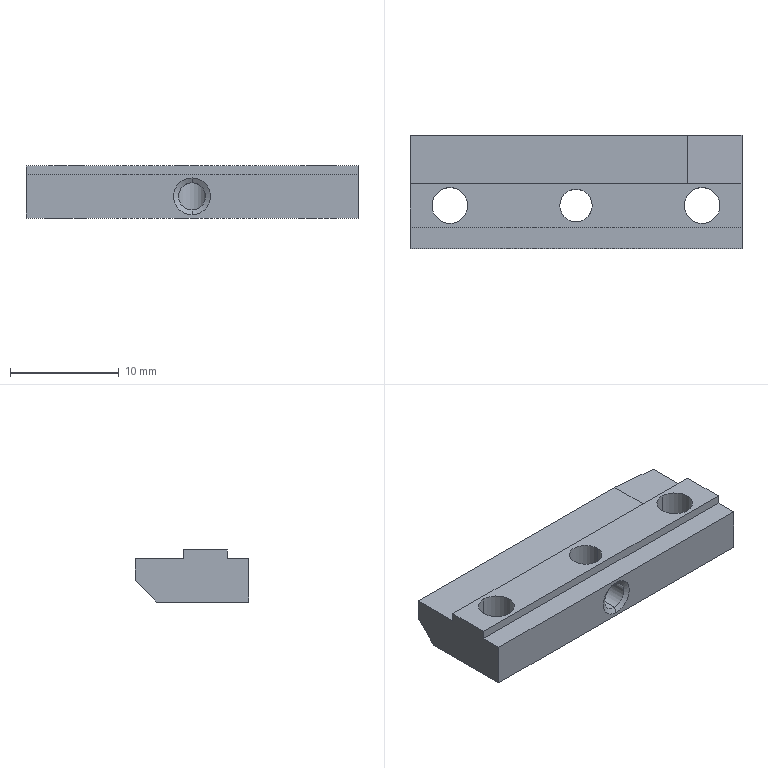Part | NX | 1 solid | 26 faces | box 30.6 x 10.5 x 4.8 mm | volume 1187 mm3 | plane 12 | cylinder 8 | cone 6 | commonest cylinder face diameters 3.3 x4 2.5 x2 3 x2
STEP:
#1=CARTESIAN_POINT('',(-174.8,180.7,-95.7));
#2=VERTEX_POINT('',#1);
#3=CARTESIAN_POINT('',(-174.8,176.706,-95.7));
#4=VERTEX_POINT('',#3);
#5=CARTESIAN_POINT('',(-174.8,178.513,-95.7));
#6=DIRECTION('',(0.,-1.,0.));
#7=VECTOR('',#6,1000.);
#8=LINE('',#5,#7);
#9=EDGE_CURVE('',#2,#4,#8,.T.);
#10=ORIENTED_EDGE('',*,*,#9,.T.);
#11=CARTESIAN_POINT('',(-144.2,176.706,-95.7));
#12=VERTEX_POINT('',#11);
#13=CARTESIAN_POINT('',(-175.,176.706,-95.7));
#14=DIRECTION('',(-1.,0.,0.));
#15=VECTOR('',#14,1000.);
#16=LINE('',#13,#15);
#17=EDGE_CURVE('',#12,#4,#16,.T.);
#18=ORIENTED_EDGE('',*,*,#17,.F.);
#19=CARTESIAN_POINT('',(-144.2,180.7,-95.7));
#20=VERTEX_POINT('',#19);
#21=CARTESIAN_POINT('',(-144.2,178.513,-95.7));
#22=DIRECTION('',(0.,-1.,0.));
#23=VECTOR('',#22,1000.);
#24=LINE('',#21,#23);
#25=EDGE_CURVE('',#20,#12,#24,.T.);
#26=ORIENTED_EDGE('',*,*,#25,.F.);
#27=CARTESIAN_POINT('',(-175.,180.7,-95.7));
#28=DIRECTION('',(1.,0.,0.));
#29=VECTOR('',#28,1000.);
#30=LINE('',#27,#29);
#31=EDGE_CURVE('',#2,#20,#30,.T.);
#32=ORIENTED_EDGE('',*,*,#31,.F.);
#33=EDGE_LOOP('',(#10,#18,#26,#32));
#34=FACE_BOUND('',#33,.T.);
#35=CARTESIAN_POINT('',(-171.125,177.05,-95.7));
#36=VERTEX_POINT('',#35);
#37=CARTESIAN_POINT('',(-171.125,180.35,-95.7));
#38=VERTEX_POINT('',#37);
#39=CARTESIAN_POINT('',(-171.125,178.7,-95.7));
#40=DIRECTION('',(0.,0.,-1.));
#41=DIRECTION('',(0.,1.,0.));
#42=AXIS2_PLACEMENT_3D('',#39,#40,#41);
#43=CIRCLE('',#42,1.65);
#44=EDGE_CURVE('',#36,#38,#43,.T.);
#45=ORIENTED_EDGE('',*,*,#44,.T.);
#46=CARTESIAN_POINT('',(-171.125,178.7,-95.7));
#47=DIRECTION('',(0.,0.,-1.));
#48=DIRECTION('',(0.,1.,0.));
#49=AXIS2_PLACEMENT_3D('',#46,#47,#48);
#50=CIRCLE('',#49,1.65);
#51=EDGE_CURVE('',#38,#36,#50,.T.);
#52=ORIENTED_EDGE('',*,*,#51,.T.);
#53=EDGE_LOOP('',(#45,#52));
#54=FACE_BOUND('',#53,.T.);
#55=CARTESIAN_POINT('',(-158.,178.7,-95.7));
#56=VERTEX_POINT('',#55);
#57=CARTESIAN_POINT('',(-161.,178.7,-95.7));
#58=VERTEX_POINT('',#57);
#59=CARTESIAN_POINT('',(-159.5,178.7,-95.7));
#60=DIRECTION('',(0.,0.,-1.));
#61=DIRECTION('',(-1.,0.,0.));
#62=AXIS2_PLACEMENT_3D('',#59,#60,#61);
#63=CIRCLE('',#62,1.5);
#64=EDGE_CURVE('',#56,#58,#63,.T.);
#65=ORIENTED_EDGE('',*,*,#64,.T.);
#66=CARTESIAN_POINT('',(-159.5,178.7,-95.7));
#67=DIRECTION('',(0.,0.,-1.));
#68=DIRECTION('',(-1.,0.,0.));
#69=AXIS2_PLACEMENT_3D('',#66,#67,#68);
#70=CIRCLE('',#69,1.5);
#71=EDGE_CURVE('',#58,#56,#70,.T.);
#72=ORIENTED_EDGE('',*,*,#71,.T.);
#73=EDGE_LOOP('',(#65,#72));
#74=FACE_BOUND('',#73,.T.);
#75=CARTESIAN_POINT('',(-147.875,177.05,-95.7));
#76=VERTEX_POINT('',#75);
#77=CARTESIAN_POINT('',(-147.875,180.35,-95.7));
#78=VERTEX_POINT('',#77);
#79=CARTESIAN_POINT('',(-147.875,178.7,-95.7));
#80=DIRECTION('',(0.,0.,-1.));
#81=DIRECTION('',(0.,1.,0.));
#82=AXIS2_PLACEMENT_3D('',#79,#80,#81);
#83=CIRCLE('',#82,1.65);
#84=EDGE_CURVE('',#76,#78,#83,.T.);
#85=ORIENTED_EDGE('',*,*,#84,.T.);
#86=CARTESIAN_POINT('',(-147.875,178.7,-95.7));
#87=DIRECTION('',(0.,0.,-1.));
#88=DIRECTION('',(0.,1.,0.));
#89=AXIS2_PLACEMENT_3D('',#86,#87,#88);
#90=CIRCLE('',#89,1.65);
#91=EDGE_CURVE('',#78,#76,#90,.T.);
#92=ORIENTED_EDGE('',*,*,#91,.T.);
#93=EDGE_LOOP('',(#85,#92));
#94=FACE_BOUND('',#93,.T.);
#95=CARTESIAN_POINT('',(-175.,176.707,-95.7));
#96=DIRECTION('',(0.,0.,1.));
#97=DIRECTION('',(1.,0.,0.));
#98=AXIS2_PLACEMENT_3D('',#95,#96,#97);
#99=PLANE('',#98);
#100=ADVANCED_FACE('',(#34,#54,#74,#94),#99,.T.);
#101=CARTESIAN_POINT('',(-174.8,176.7,-96.5));
#102=VERTEX_POINT('',#101);
#103=CARTESIAN_POINT('',(-174.8,176.744,-90.15));
#104=DIRECTION('',(0.,-0.007004,-1.));
#105=VECTOR('',#104,1000.);
#106=LINE('',#103,#105);
#107=EDGE_CURVE('',#4,#102,#106,.T.);
#108=ORIENTED_EDGE('',*,*,#107,.T.);
#109=CARTESIAN_POINT('',(-144.2,176.7,-96.5));
#110=VERTEX_POINT('',#109);
#111=CARTESIAN_POINT('',(-175.,176.7,-96.5));
#112=DIRECTION('',(1.,0.,0.));
#113=VECTOR('',#112,1000.);
#114=LINE('',#111,#113);
#115=EDGE_CURVE('',#102,#110,#114,.T.);
#116=ORIENTED_EDGE('',*,*,#115,.T.);
#117=CARTESIAN_POINT('',(-144.2,176.744,-90.15));
#118=DIRECTION('',(0.,-0.007004,-1.));
#119=VECTOR('',#118,1000.);
#120=LINE('',#117,#119);
#121=EDGE_CURVE('',#12,#110,#120,.T.);
#122=ORIENTED_EDGE('',*,*,#121,.F.);
#123=ORIENTED_EDGE('',*,*,#17,.T.);
#124=EDGE_LOOP('',(#108,#116,#122,#123));
#125=FACE_BOUND('',#124,.T.);
#126=CARTESIAN_POINT('',(-175.,176.7,-96.5));
#127=DIRECTION('',(0.,-1.,0.007004));
#128=DIRECTION('',(-1.,0.,0.));
#129=AXIS2_PLACEMENT_3D('',#126,#127,#128);
#130=PLANE('',#129);
#131=ADVANCED_FACE('',(#125),#130,.T.);
#132=CARTESIAN_POINT('',(-174.8,174.7,-96.5));
#133=VERTEX_POINT('',#132);
#134=CARTESIAN_POINT('',(-174.8,178.513,-96.5));
#135=DIRECTION('',(0.,-1.,0.));
#136=VECTOR('',#135,1000.);
#137=LINE('',#134,#136);
#138=EDGE_CURVE('',#102,#133,#137,.T.);
#139=ORIENTED_EDGE('',*,*,#138,.T.);
#140=CARTESIAN_POINT('',(-144.2,174.7,-96.5));
#141=VERTEX_POINT('',#140);
#142=CARTESIAN_POINT('',(-175.,174.7,-96.5));
#143=DIRECTION('',(1.,0.,0.));
#144=VECTOR('',#143,1000.);
#145=LINE('',#142,#144);
#146=EDGE_CURVE('',#133,#141,#145,.T.);
#147=ORIENTED_EDGE('',*,*,#146,.T.);
#148=CARTESIAN_POINT('',(-144.2,178.513,-96.5));
#149=DIRECTION('',(0.,-1.,0.));
#150=VECTOR('',#149,1000.);
#151=LINE('',#148,#150);
#152=EDGE_CURVE('',#110,#141,#151,.T.);
#153=ORIENTED_EDGE('',*,*,#152,.F.);
#154=ORIENTED_EDGE('',*,*,#115,.F.);
#155=EDGE_LOOP('',(#139,#147,#153,#154));
#156=FACE_BOUND('',#155,.T.);
#157=CARTESIAN_POINT('',(-175.,174.7,-96.5));
#158=DIRECTION('',(0.,0.,1.));
#159=DIRECTION('',(1.,0.,0.));
#160=AXIS2_PLACEMENT_3D('',#157,#158,#159);
#161=PLANE('',#160);
#162=ADVANCED_FACE('',(#156),#161,.T.);
#163=CARTESIAN_POINT('',(-174.8,174.7,-100.5));
#164=VERTEX_POINT('',#163);
#165=CARTESIAN_POINT('',(-174.8,174.7,-90.15));
#166=DIRECTION('',(0.,0.,-1.));
#167=VECTOR('',#166,1000.);
#168=LINE('',#165,#167);
#169=EDGE_CURVE('',#133,#164,#168,.T.);
#170=ORIENTED_EDGE('',*,*,#169,.T.);
#171=CARTESIAN_POINT('',(-144.2,174.7,-100.5));
#172=VERTEX_POINT('',#171);
#173=CARTESIAN_POINT('',(-175.,174.7,-100.5));
#174=DIRECTION('',(1.,0.,0.));
#175=VECTOR('',#174,1000.);
#176=LINE('',#173,#175);
#177=EDGE_CURVE('',#164,#172,#176,.T.);
#178=ORIENTED_EDGE('',*,*,#177,.T.);
#179=CARTESIAN_POINT('',(-144.2,174.7,-90.15));
#180=DIRECTION('',(0.,0.,-1.));
#181=VECTOR('',#180,1000.);
#182=LINE('',#179,#181);
#183=EDGE_CURVE('',#141,#172,#182,.T.);
#184=ORIENTED_EDGE('',*,*,#183,.F.);
#185=ORIENTED_EDGE('',*,*,#146,.F.);
#186=EDGE_LOOP('',(#170,#178,#184,#185));
#187=FACE_BOUND('',#186,.T.);
#188=CARTESIAN_POINT('',(-159.5,174.7,-96.8));
#189=VERTEX_POINT('',#188);
#190=CARTESIAN_POINT('',(-159.5,174.7,-100.2));
#191=VERTEX_POINT('',#190);
#192=CARTESIAN_POINT('',(-159.5,174.7,-98.5));
#193=DIRECTION('',(0.,-1.,0.));
#194=DIRECTION('',(0.,0.,-1.));
#195=AXIS2_PLACEMENT_3D('',#192,#193,#194);
#196=CIRCLE('',#195,1.7);
#197=EDGE_CURVE('',#189,#191,#196,.T.);
#198=ORIENTED_EDGE('',*,*,#197,.F.);
#199=CARTESIAN_POINT('',(-159.5,174.7,-98.5));
#200=DIRECTION('',(0.,-1.,0.));
#201=DIRECTION('',(0.,0.,-1.));
#202=AXIS2_PLACEMENT_3D('',#199,#200,#201);
#203=CIRCLE('',#202,1.7);
#204=EDGE_CURVE('',#191,#189,#203,.T.);
#205=ORIENTED_EDGE('',*,*,#204,.F.);
#206=EDGE_LOOP('',(#198,#205));
#207=FACE_BOUND('',#206,.T.);
#208=CARTESIAN_POINT('',(-175.,174.7,-100.5));
#209=DIRECTION('',(0.,-1.,0.));
#210=DIRECTION('',(-1.,0.,0.));
#211=AXIS2_PLACEMENT_3D('',#208,#209,#210);
#212=PLANE('',#211);
#213=ADVANCED_FACE('',(#187,#207),#212,.T.);
#214=CARTESIAN_POINT('',(-174.8,183.2,-100.5));
#215=VERTEX_POINT('',#214);
#216=CARTESIAN_POINT('',(-144.2,183.2,-100.5));
#217=VERTEX_POINT('',#216);
#218=CARTESIAN_POINT('',(-175.,183.2,-100.5));
#219=DIRECTION('',(1.,0.,0.));
#220=VECTOR('',#219,1000.);
#221=LINE('',#218,#220);
#222=EDGE_CURVE('',#215,#217,#221,.T.);
#223=ORIENTED_EDGE('',*,*,#222,.T.);
#224=CARTESIAN_POINT('',(-144.2,178.513,-100.5));
#225=DIRECTION('',(0.,1.,0.));
#226=VECTOR('',#225,1000.);
#227=LINE('',#224,#226);
#228=EDGE_CURVE('',#172,#217,#227,.T.);
#229=ORIENTED_EDGE('',*,*,#228,.F.);
#230=ORIENTED_EDGE('',*,*,#177,.F.);
#231=CARTESIAN_POINT('',(-174.8,178.513,-100.5));
#232=DIRECTION('',(0.,1.,0.));
#233=VECTOR('',#232,1000.);
#234=LINE('',#231,#233);
#235=EDGE_CURVE('',#164,#215,#234,.T.);
#236=ORIENTED_EDGE('',*,*,#235,.T.);
#237=EDGE_LOOP('',(#223,#229,#230,#236));
#238=FACE_BOUND('',#237,.T.);
#239=CARTESIAN_POINT('',(-147.875,176.85,-100.5));
#240=VERTEX_POINT('',#239);
#241=CARTESIAN_POINT('',(-147.875,180.55,-100.5));
#242=VERTEX_POINT('',#241);
#243=CARTESIAN_POINT('',(-147.875,178.7,-100.5));
#244=DIRECTION('',(0.,0.,-1.));
#245=DIRECTION('',(0.,1.,0.));
#246=AXIS2_PLACEMENT_3D('',#243,#244,#245);
#247=CIRCLE('',#246,1.85);
#248=EDGE_CURVE('',#240,#242,#247,.T.);
#249=ORIENTED_EDGE('',*,*,#248,.F.);
#250=CARTESIAN_POINT('',(-147.875,178.7,-100.5));
#251=DIRECTION('',(0.,0.,-1.));
#252=DIRECTION('',(0.,1.,0.));
#253=AXIS2_PLACEMENT_3D('',#250,#251,#252);
#254=CIRCLE('',#253,1.85);
#255=EDGE_CURVE('',#242,#240,#254,.T.);
#256=ORIENTED_EDGE('',*,*,#255,.F.);
#257=EDGE_LOOP('',(#249,#256));
#258=FACE_BOUND('',#257,.T.);
#259=CARTESIAN_POINT('',(-158.,178.7,-100.5));
#260=VERTEX_POINT('',#259);
#261=CARTESIAN_POINT('',(-161.,178.7,-100.5));
#262=VERTEX_POINT('',#261);
#263=CARTESIAN_POINT('',(-159.5,178.7,-100.5));
#264=DIRECTION('',(0.,0.,-1.));
#265=DIRECTION('',(-1.,0.,0.));
#266=AXIS2_PLACEMENT_3D('',#263,#264,#265);
#267=CIRCLE('',#266,1.5);
#268=EDGE_CURVE('',#260,#262,#267,.T.);
#269=ORIENTED_EDGE('',*,*,#268,.F.);
#270=CARTESIAN_POINT('',(-159.5,178.7,-100.5));
#271=DIRECTION('',(0.,0.,-1.));
#272=DIRECTION('',(-1.,0.,0.));
#273=AXIS2_PLACEMENT_3D('',#270,#271,#272);
#274=CIRCLE('',#273,1.5);
#275=EDGE_CURVE('',#262,#260,#274,.T.);
#276=ORIENTED_EDGE('',*,*,#275,.F.);
#277=EDGE_LOOP('',(#269,#276));
#278=FACE_BOUND('',#277,.T.);
#279=CARTESIAN_POINT('',(-171.125,176.85,-100.5));
#280=VERTEX_POINT('',#279);
#281=CARTESIAN_POINT('',(-171.125,180.55,-100.5));
#282=VERTEX_POINT('',#281);
#283=CARTESIAN_POINT('',(-171.125,178.7,-100.5));
#284=DIRECTION('',(0.,0.,-1.));
#285=DIRECTION('',(0.,1.,0.));
#286=AXIS2_PLACEMENT_3D('',#283,#284,#285);
#287=CIRCLE('',#286,1.85);
#288=EDGE_CURVE('',#280,#282,#287,.T.);
#289=ORIENTED_EDGE('',*,*,#288,.F.);
#290=CARTESIAN_POINT('',(-171.125,178.7,-100.5));
#291=DIRECTION('',(0.,0.,-1.));
#292=DIRECTION('',(0.,1.,0.));
#293=AXIS2_PLACEMENT_3D('',#290,#291,#292);
#294=CIRCLE('',#293,1.85);
#295=EDGE_CURVE('',#282,#280,#294,.T.);
#296=ORIENTED_EDGE('',*,*,#295,.F.);
#297=EDGE_LOOP('',(#289,#296));
#298=FACE_BOUND('',#297,.T.);
#299=CARTESIAN_POINT('',(-175.,182.7,-100.5));
#300=DIRECTION('',(0.,0.,-1.));
#301=DIRECTION('',(-1.,0.,0.));
#302=AXIS2_PLACEMENT_3D('',#299,#300,#301);
#303=PLANE('',#302);
#304=ADVANCED_FACE('',(#238,#258,#278,#298),#303,.T.);
#305=CARTESIAN_POINT('',(-174.8,185.2,-98.5));
#306=VERTEX_POINT('',#305);
#307=CARTESIAN_POINT('',(-174.8,185.2,-96.5));
#308=VERTEX_POINT('',#307);
#309=CARTESIAN_POINT('',(-174.8,185.2,-90.15));
#310=DIRECTION('',(0.,0.,1.));
#311=VECTOR('',#310,1000.);
#312=LINE('',#309,#311);
#313=EDGE_CURVE('',#306,#308,#312,.T.);
#314=ORIENTED_EDGE('',*,*,#313,.T.);
#315=CARTESIAN_POINT('',(-149.2,185.2,-96.5));
#316=VERTEX_POINT('',#315);
#317=CARTESIAN_POINT('',(-175.,185.2,-96.5));
#318=DIRECTION('',(-1.,0.,0.));
#319=VECTOR('',#318,1000.);
#320=LINE('',#317,#319);
#321=EDGE_CURVE('',#316,#308,#320,.T.);
#322=ORIENTED_EDGE('',*,*,#321,.F.);
#323=CARTESIAN_POINT('',(-144.2,185.2,-96.937));
#324=VERTEX_POINT('',#323);
#325=CARTESIAN_POINT('',(-175.,185.2,-94.243));
#326=DIRECTION('',(-0.9962,0.,0.08716));
#327=VECTOR('',#326,1000.);
#328=LINE('',#325,#327);
#329=EDGE_CURVE('',#324,#316,#328,.T.);
#330=ORIENTED_EDGE('',*,*,#329,.F.);
#331=CARTESIAN_POINT('',(-144.2,185.2,-98.5));
#332=VERTEX_POINT('',#331);
#333=CARTESIAN_POINT('',(-144.2,185.2,-90.15));
#334=DIRECTION('',(0.,0.,1.));
#335=VECTOR('',#334,1000.);
#336=LINE('',#333,#335);
#337=EDGE_CURVE('',#332,#324,#336,.T.);
#338=ORIENTED_EDGE('',*,*,#337,.F.);
#339=CARTESIAN_POINT('',(-175.,185.2,-98.5));
#340=DIRECTION('',(1.,0.,0.));
#341=VECTOR('',#340,1000.);
#342=LINE('',#339,#341);
#343=EDGE_CURVE('',#306,#332,#342,.T.);
#344=ORIENTED_EDGE('',*,*,#343,.F.);
#345=EDGE_LOOP('',(#314,#322,#330,#338,#344));
#346=FACE_BOUND('',#345,.T.);
#347=CARTESIAN_POINT('',(-175.,185.2,-96.5));
#348=DIRECTION('',(0.,1.,0.));
#349=DIRECTION('',(1.,0.,0.));
#350=AXIS2_PLACEMENT_3D('',#347,#348,#349);
#351=PLANE('',#350);
#352=ADVANCED_FACE('',(#346),#351,.T.);
#353=CARTESIAN_POINT('',(-174.8,180.7,-96.5));
#354=VERTEX_POINT('',#353);
#355=CARTESIAN_POINT('',(-174.8,178.513,-96.5));
#356=DIRECTION('',(0.,-1.,0.));
#357=VECTOR('',#356,1000.);
#358=LINE('',#355,#357);
#359=EDGE_CURVE('',#308,#354,#358,.T.);
#360=ORIENTED_EDGE('',*,*,#359,.T.);
#361=CARTESIAN_POINT('',(-149.2,180.7,-96.5));
#362=VERTEX_POINT('',#361);
#363=CARTESIAN_POINT('',(-175.,180.7,-96.5));
#364=DIRECTION('',(1.,0.,0.));
#365=VECTOR('',#364,1000.);
#366=LINE('',#363,#365);
#367=EDGE_CURVE('',#354,#362,#366,.T.);
#368=ORIENTED_EDGE('',*,*,#367,.T.);
#369=CARTESIAN_POINT('',(-149.2,182.95,-96.5));
#370=DIRECTION('',(0.,-1.,0.));
#371=VECTOR('',#370,1000.);
#372=LINE('',#369,#371);
#373=EDGE_CURVE('',#316,#362,#372,.T.);
#374=ORIENTED_EDGE('',*,*,#373,.F.);
#375=ORIENTED_EDGE('',*,*,#321,.T.);
#376=EDGE_LOOP('',(#360,#368,#374,#375));
#377=FACE_BOUND('',#376,.T.);
#378=CARTESIAN_POINT('',(-175.,180.7,-96.5));
#379=DIRECTION('',(0.,0.,1.));
#380=DIRECTION('',(1.,0.,0.));
#381=AXIS2_PLACEMENT_3D('',#378,#379,#380);
#382=PLANE('',#381);
#383=ADVANCED_FACE('',(#377),#382,.T.);
#384=CARTESIAN_POINT('',(-174.8,180.7,-90.15));
#385=DIRECTION('',(0.,0.,1.));
#386=VECTOR('',#385,1000.);
#387=LINE('',#384,#386);
#388=EDGE_CURVE('',#354,#2,#387,.T.);
#389=ORIENTED_EDGE('',*,*,#388,.T.);
#390=ORIENTED_EDGE('',*,*,#31,.T.);
#391=CARTESIAN_POINT('',(-144.2,180.7,-96.937));
#392=VERTEX_POINT('',#391);
#393=CARTESIAN_POINT('',(-144.2,180.7,-90.15));
#394=DIRECTION('',(0.,0.,1.));
#395=VECTOR('',#394,1000.);
#396=LINE('',#393,#395);
#397=EDGE_CURVE('',#392,#20,#396,.T.);
#398=ORIENTED_EDGE('',*,*,#397,.F.);
#399=CARTESIAN_POINT('',(-175.,180.7,-94.243));
#400=DIRECTION('',(-0.9962,0.,0.08716));
#401=VECTOR('',#400,1000.);
#402=LINE('',#399,#401);
#403=EDGE_CURVE('',#392,#362,#402,.T.);
#404=ORIENTED_EDGE('',*,*,#403,.T.);
#405=ORIENTED_EDGE('',*,*,#367,.F.);
#406=EDGE_LOOP('',(#389,#390,#398,#404,#405));
#407=FACE_BOUND('',#406,.T.);
#408=CARTESIAN_POINT('',(-175.,180.7,-95.5));
#409=DIRECTION('',(0.,1.,0.));
#410=DIRECTION('',(1.,0.,0.));
#411=AXIS2_PLACEMENT_3D('',#408,#409,#410);
#412=PLANE('',#411);
#413=ADVANCED_FACE('',(#407),#412,.T.);
#414=CARTESIAN_POINT('',(-171.125,177.05,-100.3));
#415=VERTEX_POINT('',#414);
#416=CARTESIAN_POINT('',(-171.125,180.35,-100.3));
#417=VERTEX_POINT('',#416);
#418=CARTESIAN_POINT('',(-171.125,178.7,-100.3));
#419=DIRECTION('',(0.,0.,-1.));
#420=DIRECTION('',(0.,1.,0.));
#421=AXIS2_PLACEMENT_3D('',#418,#419,#420);
#422=CIRCLE('',#421,1.65);
#423=EDGE_CURVE('',#415,#417,#422,.T.);
#424=ORIENTED_EDGE('',*,*,#423,.T.);
#425=CARTESIAN_POINT('',(-171.125,180.35,-100.5));
#426=DIRECTION('',(0.,0.,-1.));
#427=VECTOR('',#426,1000.);
#428=LINE('',#425,#427);
#429=EDGE_CURVE('',#417,#38,#428,.F.);
#430=ORIENTED_EDGE('',*,*,#429,.T.);
#431=ORIENTED_EDGE('',*,*,#44,.F.);
#432=CARTESIAN_POINT('',(-171.125,177.05,-100.5));
#433=DIRECTION('',(0.,0.,-1.));
#434=VECTOR('',#433,1000.);
#435=LINE('',#432,#434);
#436=EDGE_CURVE('',#415,#36,#435,.F.);
#437=ORIENTED_EDGE('',*,*,#436,.F.);
#438=EDGE_LOOP('',(#424,#430,#431,#437));
#439=FACE_BOUND('',#438,.T.);
#440=CARTESIAN_POINT('',(-171.125,178.7,-100.5));
#441=DIRECTION('',(0.,0.,-1.));
#442=DIRECTION('',(0.,1.,0.));
#443=AXIS2_PLACEMENT_3D('',#440,#441,#442);
#444=CYLINDRICAL_SURFACE('',#443,1.65);
#445=ADVANCED_FACE('',(#439),#444,.F.);
#446=ORIENTED_EDGE('',*,*,#423,.F.);
#447=CARTESIAN_POINT('',(-171.125,177.05,-100.3));
#448=DIRECTION('',(0.,-0.7071,-0.7071));
#449=VECTOR('',#448,1000.);
#450=LINE('',#447,#449);
#451=EDGE_CURVE('',#280,#415,#450,.F.);
#452=ORIENTED_EDGE('',*,*,#451,.F.);
#453=ORIENTED_EDGE('',*,*,#288,.T.);
#454=CARTESIAN_POINT('',(-171.125,180.35,-100.3));
#455=DIRECTION('',(0.,0.7071,-0.7071));
#456=VECTOR('',#455,1000.);
#457=LINE('',#454,#456);
#458=EDGE_CURVE('',#282,#417,#457,.F.);
#459=ORIENTED_EDGE('',*,*,#458,.T.);
#460=EDGE_LOOP('',(#446,#452,#453,#459));
#461=FACE_BOUND('',#460,.T.);
#462=CARTESIAN_POINT('',(-171.125,178.7,-100.3));
#463=DIRECTION('',(0.,0.,-1.));
#464=DIRECTION('',(0.,1.,0.));
#465=AXIS2_PLACEMENT_3D('',#462,#463,#464);
#466=CONICAL_SURFACE('',#465,1.65,0.7854);
#467=ADVANCED_FACE('',(#461),#466,.F.);
#468=CARTESIAN_POINT('',(-147.875,177.05,-100.3));
#469=VERTEX_POINT('',#468);
#470=CARTESIAN_POINT('',(-147.875,180.35,-100.3));
#471=VERTEX_POINT('',#470);
#472=CARTESIAN_POINT('',(-147.875,178.7,-100.3));
#473=DIRECTION('',(0.,0.,-1.));
#474=DIRECTION('',(0.,1.,0.));
#475=AXIS2_PLACEMENT_3D('',#472,#473,#474);
#476=CIRCLE('',#475,1.65);
#477=EDGE_CURVE('',#469,#471,#476,.T.);
#478=ORIENTED_EDGE('',*,*,#477,.T.);
#479=CARTESIAN_POINT('',(-147.875,180.35,-100.5));
#480=DIRECTION('',(0.,0.,-1.));
#481=VECTOR('',#480,1000.);
#482=LINE('',#479,#481);
#483=EDGE_CURVE('',#471,#78,#482,.F.);
#484=ORIENTED_EDGE('',*,*,#483,.T.);
#485=ORIENTED_EDGE('',*,*,#84,.F.);
#486=CARTESIAN_POINT('',(-147.875,177.05,-100.5));
#487=DIRECTION('',(0.,0.,-1.));
#488=VECTOR('',#487,1000.);
#489=LINE('',#486,#488);
#490=EDGE_CURVE('',#469,#76,#489,.F.);
#491=ORIENTED_EDGE('',*,*,#490,.F.);
#492=EDGE_LOOP('',(#478,#484,#485,#491));
#493=FACE_BOUND('',#492,.T.);
#494=CARTESIAN_POINT('',(-147.875,178.7,-100.5));
#495=DIRECTION('',(0.,0.,-1.));
#496=DIRECTION('',(0.,1.,0.));
#497=AXIS2_PLACEMENT_3D('',#494,#495,#496);
#498=CYLINDRICAL_SURFACE('',#497,1.65);
#499=ADVANCED_FACE('',(#493),#498,.F.);
#500=ORIENTED_EDGE('',*,*,#477,.F.);
#501=CARTESIAN_POINT('',(-147.875,177.05,-100.3));
#502=DIRECTION('',(0.,-0.7071,-0.7071));
#503=VECTOR('',#502,1000.);
#504=LINE('',#501,#503);
#505=EDGE_CURVE('',#240,#469,#504,.F.);
#506=ORIENTED_EDGE('',*,*,#505,.F.);
#507=ORIENTED_EDGE('',*,*,#248,.T.);
#508=CARTESIAN_POINT('',(-147.875,180.35,-100.3));
#509=DIRECTION('',(0.,0.7071,-0.7071));
#510=VECTOR('',#509,1000.);
#511=LINE('',#508,#510);
#512=EDGE_CURVE('',#242,#471,#511,.F.);
#513=ORIENTED_EDGE('',*,*,#512,.T.);
#514=EDGE_LOOP('',(#500,#506,#507,#513));
#515=FACE_BOUND('',#514,.T.);
#516=CARTESIAN_POINT('',(-147.875,178.7,-100.3));
#517=DIRECTION('',(0.,0.,-1.));
#518=DIRECTION('',(0.,1.,0.));
#519=AXIS2_PLACEMENT_3D('',#516,#517,#518);
#520=CONICAL_SURFACE('',#519,1.65,0.7854);
#521=ADVANCED_FACE('',(#515),#520,.F.);
#522=ORIENTED_EDGE('',*,*,#64,.F.);
#523=CARTESIAN_POINT('',(-158.,178.7,-95.22));
#524=DIRECTION('',(0.,0.,-1.));
#525=VECTOR('',#524,1000.);
#526=LINE('',#523,#525);
#527=EDGE_CURVE('',#260,#56,#526,.F.);
#528=ORIENTED_EDGE('',*,*,#527,.F.);
#529=ORIENTED_EDGE('',*,*,#268,.T.);
#530=CARTESIAN_POINT('',(-161.,178.7,-95.22));
#531=DIRECTION('',(0.,0.,-1.));
#532=VECTOR('',#531,1000.);
#533=LINE('',#530,#532);
#534=EDGE_CURVE('',#262,#58,#533,.F.);
#535=ORIENTED_EDGE('',*,*,#534,.T.);
#536=EDGE_LOOP('',(#522,#528,#529,#535));
#537=FACE_BOUND('',#536,.T.);
#538=CARTESIAN_POINT('',(-159.5,177.2,-97.25));
#539=VERTEX_POINT('',#538);
#540=CARTESIAN_POINT('',(-160.75,177.871,-98.5));
#541=VERTEX_POINT('',#540);
#542=CARTESIAN_POINT('',(-159.5,177.2,-97.25));
#543=CARTESIAN_POINT('',(-159.522,177.2,-97.25));
#544=CARTESIAN_POINT('',(-159.544,177.2,-97.251));
#545=CARTESIAN_POINT('',(-159.566,177.201,-97.252));
#546=CARTESIAN_POINT('',(-159.587,177.202,-97.253));
#547=CARTESIAN_POINT('',(-159.609,177.204,-97.255));
#548=CARTESIAN_POINT('',(-159.631,177.206,-97.257));
#549=CARTESIAN_POINT('',(-159.653,177.208,-97.259));
#550=CARTESIAN_POINT('',(-159.674,177.21,-97.262));
#551=CARTESIAN_POINT('',(-159.696,177.213,-97.265));
#552=CARTESIAN_POINT('',(-159.717,177.216,-97.269));
#553=CARTESIAN_POINT('',(-159.738,177.219,-97.273));
#554=CARTESIAN_POINT('',(-159.759,177.223,-97.277));
#555=CARTESIAN_POINT('',(-159.78,177.226,-97.282));
#556=CARTESIAN_POINT('',(-159.801,177.23,-97.287));
#557=CARTESIAN_POINT('',(-159.822,177.235,-97.292));
#558=CARTESIAN_POINT('',(-159.842,177.239,-97.298));
#559=CARTESIAN_POINT('',(-159.863,177.244,-97.304));
#560=CARTESIAN_POINT('',(-159.883,177.25,-97.31));
#561=CARTESIAN_POINT('',(-159.903,177.255,-97.317));
#562=CARTESIAN_POINT('',(-159.923,177.261,-97.324));
#563=CARTESIAN_POINT('',(-159.943,177.267,-97.331));
#564=CARTESIAN_POINT('',(-159.962,177.273,-97.338));
#565=CARTESIAN_POINT('',(-159.982,177.279,-97.346));
#566=CARTESIAN_POINT('',(-160.001,177.286,-97.355));
#567=CARTESIAN_POINT('',(-160.02,177.293,-97.363));
#568=CARTESIAN_POINT('',(-160.039,177.3,-97.372));
#569=CARTESIAN_POINT('',(-160.057,177.307,-97.381));
#570=CARTESIAN_POINT('',(-160.076,177.315,-97.39));
#571=CARTESIAN_POINT('',(-160.094,177.322,-97.4));
#572=CARTESIAN_POINT('',(-160.111,177.33,-97.41));
#573=CARTESIAN_POINT('',(-160.147,177.346,-97.429));
#574=CARTESIAN_POINT('',(-160.181,177.363,-97.451));
#575=CARTESIAN_POINT('',(-160.214,177.381,-97.474));
#576=CARTESIAN_POINT('',(-160.246,177.398,-97.496));
#577=CARTESIAN_POINT('',(-160.278,177.417,-97.521));
#578=CARTESIAN_POINT('',(-160.308,177.436,-97.546));
#579=CARTESIAN_POINT('',(-160.338,177.455,-97.572));
#580=CARTESIAN_POINT('',(-160.367,177.475,-97.598));
#581=CARTESIAN_POINT('',(-160.394,177.495,-97.626));
#582=CARTESIAN_POINT('',(-160.407,177.505,-97.64));
#583=CARTESIAN_POINT('',(-160.421,177.516,-97.654));
#584=CARTESIAN_POINT('',(-160.433,177.526,-97.669));
#585=CARTESIAN_POINT('',(-160.446,177.536,-97.683));
#586=CARTESIAN_POINT('',(-160.459,177.546,-97.698));
#587=CARTESIAN_POINT('',(-160.471,177.556,-97.712));
#588=CARTESIAN_POINT('',(-160.483,177.567,-97.727));
#589=CARTESIAN_POINT('',(-160.495,177.577,-97.743));
#590=CARTESIAN_POINT('',(-160.506,177.587,-97.758));
#591=CARTESIAN_POINT('',(-160.517,177.598,-97.774));
#592=CARTESIAN_POINT('',(-160.529,177.608,-97.789));
#593=CARTESIAN_POINT('',(-160.539,177.618,-97.805));
#594=CARTESIAN_POINT('',(-160.55,177.629,-97.821));
#595=CARTESIAN_POINT('',(-160.56,177.639,-97.838));
#596=CARTESIAN_POINT('',(-160.57,177.649,-97.854));
#597=CARTESIAN_POINT('',(-160.58,177.659,-97.871));
#598=CARTESIAN_POINT('',(-160.59,177.669,-97.888));
#599=CARTESIAN_POINT('',(-160.599,177.679,-97.905));
#600=CARTESIAN_POINT('',(-160.609,177.689,-97.922));
#601=CARTESIAN_POINT('',(-160.617,177.699,-97.94));
#602=CARTESIAN_POINT('',(-160.626,177.709,-97.957));
#603=CARTESIAN_POINT('',(-160.634,177.719,-97.975));
#604=CARTESIAN_POINT('',(-160.643,177.728,-97.993));
#605=CARTESIAN_POINT('',(-160.65,177.737,-98.011));
#606=CARTESIAN_POINT('',(-160.658,177.747,-98.029));
#607=CARTESIAN_POINT('',(-160.665,177.756,-98.048));
#608=CARTESIAN_POINT('',(-160.672,177.764,-98.066));
#609=CARTESIAN_POINT('',(-160.679,177.773,-98.085));
#610=CARTESIAN_POINT('',(-160.686,177.781,-98.104));
#611=CARTESIAN_POINT('',(-160.692,177.789,-98.123));
#612=CARTESIAN_POINT('',(-160.698,177.797,-98.143));
#613=CARTESIAN_POINT('',(-160.704,177.805,-98.163));
#614=CARTESIAN_POINT('',(-160.709,177.812,-98.183));
#615=CARTESIAN_POINT('',(-160.714,177.819,-98.203));
#616=CARTESIAN_POINT('',(-160.719,177.826,-98.223));
#617=CARTESIAN_POINT('',(-160.723,177.832,-98.243));
#618=CARTESIAN_POINT('',(-160.728,177.838,-98.264));
#619=CARTESIAN_POINT('',(-160.732,177.844,-98.285));
#620=CARTESIAN_POINT('',(-160.735,177.848,-98.306));
#621=CARTESIAN_POINT('',(-160.738,177.853,-98.327));
#622=CARTESIAN_POINT('',(-160.741,177.857,-98.348));
#623=CARTESIAN_POINT('',(-160.743,177.861,-98.37));
#624=CARTESIAN_POINT('',(-160.745,177.864,-98.391));
#625=CARTESIAN_POINT('',(-160.747,177.867,-98.413));
#626=CARTESIAN_POINT('',(-160.748,177.868,-98.434));
#627=CARTESIAN_POINT('',(-160.749,177.869,-98.445));
#628=CARTESIAN_POINT('',(-160.749,177.87,-98.456));
#629=CARTESIAN_POINT('',(-160.75,177.87,-98.467));
#630=CARTESIAN_POINT('',(-160.75,177.871,-98.478));
#631=CARTESIAN_POINT('',(-160.75,177.871,-98.489));
#632=CARTESIAN_POINT('',(-160.75,177.871,-98.5));
#633=B_SPLINE_CURVE_WITH_KNOTS('',3,(#542,#543,#544,#545,#546,#547,#548,#549,#550,#551,#552,#553,#554,#555,#556,#557,#558,#559,#560,#561,#562,#563,#564,#565,#566,#567,#568,#569,#570,#571,#572,#573,#574,#575,#576,#577,#578,#579,#580,#581,#582,#583,#584,#585,#586,#587,#588,#589,#590,#591,#592,#593,#594,#595,#596,#597,#598,#599,#600,#601,#602,#603,#604,#605,#606,#607,#608,#609,#610,#611,#612,#613,#614,#615,#616,#617,#618,#619,#620,#621,#622,#623,#624,#625,#626,#627,#628,#629,#630,#631,#632),.UNSPECIFIED.,.F.,.F.,(4,3,3,3,3,3,3,3,3,3,3,3,3,3,3,3,3,3,3,3,3,3,3,3,3,3,3,3,3,3,4),(0.,0.0656,0.1313,0.197,0.2625,0.3278,0.3933,0.459,0.5247,0.5903,0.6557,0.7865,0.9179,1.049,1.115,1.18,1.246,1.311,1.377,1.443,1.508,1.574,1.639,1.705,1.77,1.836,1.902,1.967,2.032,2.065,2.098),.UNSPECIFIED.);
#634=EDGE_CURVE('',#539,#541,#633,.T.);
#635=ORIENTED_EDGE('',*,*,#634,.T.);
#636=CARTESIAN_POINT('',(-159.5,177.2,-99.75));
#637=VERTEX_POINT('',#636);
#638=CARTESIAN_POINT('',(-160.75,177.871,-98.5));
#639=CARTESIAN_POINT('',(-160.75,177.871,-98.511));
#640=CARTESIAN_POINT('',(-160.75,177.871,-98.522));
#641=CARTESIAN_POINT('',(-160.75,177.87,-98.533));
#642=CARTESIAN_POINT('',(-160.749,177.87,-98.544));
#643=CARTESIAN_POINT('',(-160.749,177.869,-98.555));
#644=CARTESIAN_POINT('',(-160.748,177.868,-98.566));
#645=CARTESIAN_POINT('',(-160.748,177.867,-98.577));
#646=CARTESIAN_POINT('',(-160.747,177.866,-98.588));
#647=CARTESIAN_POINT('',(-160.746,177.865,-98.598));
#648=CARTESIAN_POINT('',(-160.745,177.864,-98.609));
#649=CARTESIAN_POINT('',(-160.744,177.862,-98.62));
#650=CARTESIAN_POINT('',(-160.743,177.861,-98.631));
#651=CARTESIAN_POINT('',(-160.741,177.857,-98.652));
#652=CARTESIAN_POINT('',(-160.738,177.853,-98.673));
#653=CARTESIAN_POINT('',(-160.735,177.848,-98.694));
#654=CARTESIAN_POINT('',(-160.732,177.844,-98.715));
#655=CARTESIAN_POINT('',(-160.728,177.838,-98.736));
#656=CARTESIAN_POINT('',(-160.723,177.832,-98.757));
#657=CARTESIAN_POINT('',(-160.719,177.826,-98.777));
#658=CARTESIAN_POINT('',(-160.714,177.819,-98.797));
#659=CARTESIAN_POINT('',(-160.709,177.812,-98.817));
#660=CARTESIAN_POINT('',(-160.704,177.805,-98.837));
#661=CARTESIAN_POINT('',(-160.698,177.797,-98.857));
#662=CARTESIAN_POINT('',(-160.692,177.789,-98.877));
#663=CARTESIAN_POINT('',(-160.686,177.781,-98.896));
#664=CARTESIAN_POINT('',(-160.679,177.773,-98.915));
#665=CARTESIAN_POINT('',(-160.672,177.764,-98.934));
#666=CARTESIAN_POINT('',(-160.665,177.756,-98.952));
#667=CARTESIAN_POINT('',(-160.658,177.747,-98.971));
#668=CARTESIAN_POINT('',(-160.65,177.737,-98.989));
#669=CARTESIAN_POINT('',(-160.643,177.728,-99.007));
#670=CARTESIAN_POINT('',(-160.635,177.719,-99.025));
#671=CARTESIAN_POINT('',(-160.626,177.709,-99.043));
#672=CARTESIAN_POINT('',(-160.618,177.699,-99.06));
#673=CARTESIAN_POINT('',(-160.609,177.69,-99.078));
#674=CARTESIAN_POINT('',(-160.599,177.68,-99.095));
#675=CARTESIAN_POINT('',(-160.59,177.67,-99.112));
#676=CARTESIAN_POINT('',(-160.581,177.659,-99.129));
#677=CARTESIAN_POINT('',(-160.571,177.649,-99.145));
#678=CARTESIAN_POINT('',(-160.561,177.639,-99.162));
#679=CARTESIAN_POINT('',(-160.55,177.629,-99.178));
#680=CARTESIAN_POINT('',(-160.539,177.619,-99.194));
#681=CARTESIAN_POINT('',(-160.529,177.608,-99.21));
#682=CARTESIAN_POINT('',(-160.518,177.598,-99.226));
#683=CARTESIAN_POINT('',(-160.506,177.588,-99.242));
#684=CARTESIAN_POINT('',(-160.495,177.577,-99.257));
#685=CARTESIAN_POINT('',(-160.483,177.567,-99.272));
#686=CARTESIAN_POINT('',(-160.471,177.557,-99.287));
#687=CARTESIAN_POINT('',(-160.447,177.536,-99.317));
#688=CARTESIAN_POINT('',(-160.421,177.516,-99.346));
#689=CARTESIAN_POINT('',(-160.394,177.496,-99.374));
#690=CARTESIAN_POINT('',(-160.367,177.475,-99.401));
#691=CARTESIAN_POINT('',(-160.338,177.456,-99.428));
#692=CARTESIAN_POINT('',(-160.308,177.436,-99.454));
#693=CARTESIAN_POINT('',(-160.278,177.417,-99.479));
#694=CARTESIAN_POINT('',(-160.247,177.398,-99.503));
#695=CARTESIAN_POINT('',(-160.214,177.381,-99.526));
#696=CARTESIAN_POINT('',(-160.181,177.363,-99.549));
#697=CARTESIAN_POINT('',(-160.147,177.346,-99.57));
#698=CARTESIAN_POINT('',(-160.111,177.33,-99.59));
#699=CARTESIAN_POINT('',(-160.076,177.314,-99.61));
#700=CARTESIAN_POINT('',(-160.039,177.3,-99.628));
#701=CARTESIAN_POINT('',(-160.001,177.286,-99.645));
#702=CARTESIAN_POINT('',(-159.982,177.279,-99.653));
#703=CARTESIAN_POINT('',(-159.963,177.273,-99.661));
#704=CARTESIAN_POINT('',(-159.943,177.267,-99.669));
#705=CARTESIAN_POINT('',(-159.923,177.261,-99.676));
#706=CARTESIAN_POINT('',(-159.903,177.255,-99.683));
#707=CARTESIAN_POINT('',(-159.883,177.25,-99.69));
#708=CARTESIAN_POINT('',(-159.863,177.244,-99.696));
#709=CARTESIAN_POINT('',(-159.842,177.239,-99.702));
#710=CARTESIAN_POINT('',(-159.822,177.235,-99.708));
#711=CARTESIAN_POINT('',(-159.801,177.23,-99.713));
#712=CARTESIAN_POINT('',(-159.78,177.226,-99.718));
#713=CARTESIAN_POINT('',(-159.759,177.223,-99.723));
#714=CARTESIAN_POINT('',(-159.738,177.219,-99.727));
#715=CARTESIAN_POINT('',(-159.717,177.216,-99.731));
#716=CARTESIAN_POINT('',(-159.695,177.213,-99.735));
#717=CARTESIAN_POINT('',(-159.674,177.21,-99.738));
#718=CARTESIAN_POINT('',(-159.653,177.208,-99.741));
#719=CARTESIAN_POINT('',(-159.631,177.206,-99.743));
#720=CARTESIAN_POINT('',(-159.609,177.204,-99.745));
#721=CARTESIAN_POINT('',(-159.587,177.202,-99.747));
#722=CARTESIAN_POINT('',(-159.566,177.201,-99.748));
#723=CARTESIAN_POINT('',(-159.544,177.2,-99.749));
#724=CARTESIAN_POINT('',(-159.522,177.2,-99.75));
#725=CARTESIAN_POINT('',(-159.5,177.2,-99.75));
#726=B_SPLINE_CURVE_WITH_KNOTS('',3,(#638,#639,#640,#641,#642,#643,#644,#645,#646,#647,#648,#649,#650,#651,#652,#653,#654,#655,#656,#657,#658,#659,#660,#661,#662,#663,#664,#665,#666,#667,#668,#669,#670,#671,#672,#673,#674,#675,#676,#677,#678,#679,#680,#681,#682,#683,#684,#685,#686,#687,#688,#689,#690,#691,#692,#693,#694,#695,#696,#697,#698,#699,#700,#701,#702,#703,#704,#705,#706,#707,#708,#709,#710,#711,#712,#713,#714,#715,#716,#717,#718,#719,#720,#721,#722,#723,#724,#725),.UNSPECIFIED.,.F.,.F.,(4,3,3,3,3,3,3,3,3,3,3,3,3,3,3,3,3,3,3,3,3,3,3,3,3,3,3,3,3,4),(0.,0.03292,0.06582,0.09866,0.1314,0.1967,0.2621,0.3278,0.3934,0.4588,0.5241,0.5895,0.6551,0.7207,0.7863,0.8519,0.9173,1.048,1.18,1.311,1.442,1.573,1.639,1.705,1.77,1.836,1.901,1.967,2.032,2.098),.UNSPECIFIED.);
#727=EDGE_CURVE('',#541,#637,#726,.T.);
#728=ORIENTED_EDGE('',*,*,#727,.T.);
#729=CARTESIAN_POINT('',(-159.5,177.2,-99.75));
#730=CARTESIAN_POINT('',(-159.472,177.2,-99.75));
#731=CARTESIAN_POINT('',(-159.445,177.201,-99.749));
#732=CARTESIAN_POINT('',(-159.417,177.202,-99.747));
#733=CARTESIAN_POINT('',(-159.402,177.203,-99.746));
#734=CARTESIAN_POINT('',(-159.387,177.204,-99.745));
#735=CARTESIAN_POINT('',(-159.372,177.205,-99.743));
#736=CARTESIAN_POINT('',(-159.357,177.207,-99.742));
#737=CARTESIAN_POINT('',(-159.342,177.208,-99.74));
#738=CARTESIAN_POINT('',(-159.327,177.21,-99.738));
#739=CARTESIAN_POINT('',(-159.297,177.213,-99.734));
#740=CARTESIAN_POINT('',(-159.268,177.218,-99.729));
#741=CARTESIAN_POINT('',(-159.239,177.223,-99.722));
#742=CARTESIAN_POINT('',(-159.209,177.228,-99.716));
#743=CARTESIAN_POINT('',(-159.18,177.234,-99.709));
#744=CARTESIAN_POINT('',(-159.152,177.241,-99.701));
#745=CARTESIAN_POINT('',(-159.123,177.248,-99.692));
#746=CARTESIAN_POINT('',(-159.096,177.255,-99.683));
#747=CARTESIAN_POINT('',(-159.068,177.263,-99.673));
#748=CARTESIAN_POINT('',(-159.041,177.272,-99.663));
#749=CARTESIAN_POINT('',(-159.014,177.281,-99.652));
#750=CARTESIAN_POINT('',(-158.988,177.29,-99.64));
#751=CARTESIAN_POINT('',(-158.962,177.3,-99.629));
#752=CARTESIAN_POINT('',(-158.936,177.31,-99.616));
#753=CARTESIAN_POINT('',(-158.911,177.32,-99.603));
#754=CARTESIAN_POINT('',(-158.886,177.331,-99.589));
#755=CARTESIAN_POINT('',(-158.862,177.342,-99.575));
#756=CARTESIAN_POINT('',(-158.838,177.354,-99.56));
#757=CARTESIAN_POINT('',(-158.814,177.366,-99.545));
#758=CARTESIAN_POINT('',(-158.791,177.378,-99.53));
#759=CARTESIAN_POINT('',(-158.768,177.391,-99.514));
#760=CARTESIAN_POINT('',(-158.743,177.404,-99.496));
#761=CARTESIAN_POINT('',(-158.719,177.419,-99.477));
#762=CARTESIAN_POINT('',(-158.696,177.434,-99.457));
#763=CARTESIAN_POINT('',(-158.673,177.448,-99.438));
#764=CARTESIAN_POINT('',(-158.651,177.463,-99.418));
#765=CARTESIAN_POINT('',(-158.629,177.479,-99.397));
#766=CARTESIAN_POINT('',(-158.608,177.494,-99.376));
#767=CARTESIAN_POINT('',(-158.587,177.51,-99.354));
#768=CARTESIAN_POINT('',(-158.567,177.526,-99.332));
#769=CARTESIAN_POINT('',(-158.547,177.541,-99.309));
#770=CARTESIAN_POINT('',(-158.528,177.557,-99.286));
#771=CARTESIAN_POINT('',(-158.51,177.573,-99.263));
#772=CARTESIAN_POINT('',(-158.491,177.589,-99.239));
#773=CARTESIAN_POINT('',(-158.474,177.606,-99.215));
#774=CARTESIAN_POINT('',(-158.458,177.621,-99.19));
#775=CARTESIAN_POINT('',(-158.441,177.637,-99.165));
#776=CARTESIAN_POINT('',(-158.425,177.653,-99.139));
#777=CARTESIAN_POINT('',(-158.411,177.669,-99.113));
#778=CARTESIAN_POINT('',(-158.403,177.677,-99.1));
#779=CARTESIAN_POINT('',(-158.396,177.684,-99.087));
#780=CARTESIAN_POINT('',(-158.389,177.692,-99.074));
#781=CARTESIAN_POINT('',(-158.382,177.699,-99.06));
#782=CARTESIAN_POINT('',(-158.376,177.707,-99.047));
#783=CARTESIAN_POINT('',(-158.369,177.714,-99.033));
#784=CARTESIAN_POINT('',(-158.356,177.729,-99.006));
#785=CARTESIAN_POINT('',(-158.344,177.743,-98.978));
#786=CARTESIAN_POINT('',(-158.333,177.757,-98.949));
#787=CARTESIAN_POINT('',(-158.327,177.765,-98.932));
#788=CARTESIAN_POINT('',(-158.321,177.773,-98.915));
#789=CARTESIAN_POINT('',(-158.315,177.781,-98.897));
#790=CARTESIAN_POINT('',(-158.309,177.788,-98.88));
#791=CARTESIAN_POINT('',(-158.303,177.795,-98.862));
#792=CARTESIAN_POINT('',(-158.298,177.802,-98.844));
#793=CARTESIAN_POINT('',(-158.288,177.816,-98.808));
#794=CARTESIAN_POINT('',(-158.279,177.828,-98.772));
#795=CARTESIAN_POINT('',(-158.272,177.838,-98.734));
#796=CARTESIAN_POINT('',(-158.269,177.844,-98.715));
#797=CARTESIAN_POINT('',(-158.265,177.848,-98.696));
#798=CARTESIAN_POINT('',(-158.263,177.852,-98.677));
#799=CARTESIAN_POINT('',(-158.26,177.856,-98.658));
#800=CARTESIAN_POINT('',(-158.258,177.86,-98.638));
#801=CARTESIAN_POINT('',(-158.256,177.862,-98.619));
#802=CARTESIAN_POINT('',(-158.254,177.865,-98.599));
#803=CARTESIAN_POINT('',(-158.252,177.867,-98.579));
#804=CARTESIAN_POINT('',(-158.251,177.869,-98.56));
#805=CARTESIAN_POINT('',(-158.25,177.87,-98.54));
#806=CARTESIAN_POINT('',(-158.25,177.871,-98.52));
#807=CARTESIAN_POINT('',(-158.25,177.871,-98.5));
#808=CARTESIAN_POINT('',(-158.25,177.871,-98.481));
#809=CARTESIAN_POINT('',(-158.25,177.87,-98.461));
#810=CARTESIAN_POINT('',(-158.251,177.869,-98.441));
#811=CARTESIAN_POINT('',(-158.252,177.867,-98.421));
#812=CARTESIAN_POINT('',(-158.254,177.865,-98.402));
#813=CARTESIAN_POINT('',(-158.256,177.862,-98.382));
#814=CARTESIAN_POINT('',(-158.257,177.86,-98.362));
#815=CARTESIAN_POINT('',(-158.26,177.856,-98.343));
#816=CARTESIAN_POINT('',(-158.263,177.852,-98.324));
#817=CARTESIAN_POINT('',(-158.265,177.848,-98.304));
#818=CARTESIAN_POINT('',(-158.268,177.844,-98.285));
#819=CARTESIAN_POINT('',(-158.272,177.839,-98.266));
#820=CARTESIAN_POINT('',(-158.274,177.836,-98.257));
#821=CARTESIAN_POINT('',(-158.276,177.833,-98.248));
#822=CARTESIAN_POINT('',(-158.278,177.831,-98.238));
#823=CARTESIAN_POINT('',(-158.28,177.828,-98.229));
#824=CARTESIAN_POINT('',(-158.282,177.825,-98.22));
#825=CARTESIAN_POINT('',(-158.284,177.822,-98.211));
#826=CARTESIAN_POINT('',(-158.288,177.816,-98.192));
#827=CARTESIAN_POINT('',(-158.293,177.809,-98.174));
#828=CARTESIAN_POINT('',(-158.298,177.802,-98.156));
#829=CARTESIAN_POINT('',(-158.303,177.796,-98.139));
#830=CARTESIAN_POINT('',(-158.309,177.788,-98.121));
#831=CARTESIAN_POINT('',(-158.315,177.781,-98.103));
#832=CARTESIAN_POINT('',(-158.32,177.773,-98.086));
#833=CARTESIAN_POINT('',(-158.327,177.766,-98.069));
#834=CARTESIAN_POINT('',(-158.333,177.757,-98.052));
#835=CARTESIAN_POINT('',(-158.344,177.744,-98.023));
#836=CARTESIAN_POINT('',(-158.356,177.729,-97.995));
#837=CARTESIAN_POINT('',(-158.369,177.715,-97.967));
#838=CARTESIAN_POINT('',(-158.376,177.707,-97.954));
#839=CARTESIAN_POINT('',(-158.382,177.7,-97.94));
#840=CARTESIAN_POINT('',(-158.389,177.692,-97.927));
#841=CARTESIAN_POINT('',(-158.396,177.684,-97.914));
#842=CARTESIAN_POINT('',(-158.403,177.677,-97.9));
#843=CARTESIAN_POINT('',(-158.41,177.669,-97.887));
#844=CARTESIAN_POINT('',(-158.425,177.654,-97.861));
#845=CARTESIAN_POINT('',(-158.441,177.638,-97.836));
#846=CARTESIAN_POINT('',(-158.457,177.622,-97.811));
#847=CARTESIAN_POINT('',(-158.474,177.606,-97.786));
#848=CARTESIAN_POINT('',(-158.491,177.59,-97.762));
#849=CARTESIAN_POINT('',(-158.509,177.574,-97.738));
#850=CARTESIAN_POINT('',(-158.527,177.558,-97.714));
#851=CARTESIAN_POINT('',(-158.547,177.542,-97.691));
#852=CARTESIAN_POINT('',(-158.566,177.526,-97.669));
#853=CARTESIAN_POINT('',(-158.586,177.51,-97.646));
#854=CARTESIAN_POINT('',(-158.607,177.494,-97.625));
#855=CARTESIAN_POINT('',(-158.629,177.479,-97.604));
#856=CARTESIAN_POINT('',(-158.65,177.464,-97.583));
#857=CARTESIAN_POINT('',(-158.673,177.448,-97.562));
#858=CARTESIAN_POINT('',(-158.696,177.434,-97.543));
#859=CARTESIAN_POINT('',(-158.707,177.426,-97.533));
#860=CARTESIAN_POINT('',(-158.719,177.419,-97.524));
#861=CARTESIAN_POINT('',(-158.731,177.412,-97.514));
#862=CARTESIAN_POINT('',(-158.743,177.405,-97.505));
#863=CARTESIAN_POINT('',(-158.756,177.398,-97.496));
#864=CARTESIAN_POINT('',(-158.768,177.391,-97.487));
#865=CARTESIAN_POINT('',(-158.79,177.378,-97.471));
#866=CARTESIAN_POINT('',(-158.814,177.366,-97.455));
#867=CARTESIAN_POINT('',(-158.837,177.354,-97.44));
#868=CARTESIAN_POINT('',(-158.861,177.343,-97.425));
#869=CARTESIAN_POINT('',(-158.886,177.331,-97.411));
#870=CARTESIAN_POINT('',(-158.911,177.321,-97.398));
#871=CARTESIAN_POINT('',(-158.936,177.31,-97.384));
#872=CARTESIAN_POINT('',(-158.962,177.3,-97.372));
#873=CARTESIAN_POINT('',(-158.988,177.29,-97.36));
#874=CARTESIAN_POINT('',(-159.014,177.281,-97.348));
#875=CARTESIAN_POINT('',(-159.041,177.272,-97.337));
#876=CARTESIAN_POINT('',(-159.068,177.264,-97.327));
#877=CARTESIAN_POINT('',(-159.082,177.259,-97.322));
#878=CARTESIAN_POINT('',(-159.095,177.256,-97.317));
#879=CARTESIAN_POINT('',(-159.109,177.252,-97.313));
#880=CARTESIAN_POINT('',(-159.123,177.248,-97.308));
#881=CARTESIAN_POINT('',(-159.137,177.244,-97.304));
#882=CARTESIAN_POINT('',(-159.151,177.241,-97.3));
#883=CARTESIAN_POINT('',(-159.18,177.234,-97.291));
#884=CARTESIAN_POINT('',(-159.209,177.228,-97.284));
#885=CARTESIAN_POINT('',(-159.238,177.223,-97.278));
#886=CARTESIAN_POINT('',(-159.253,177.22,-97.275));
#887=CARTESIAN_POINT('',(-159.267,177.218,-97.272));
#888=CARTESIAN_POINT('',(-159.282,177.216,-97.269));
#889=CARTESIAN_POINT('',(-159.297,177.214,-97.266));
#890=CARTESIAN_POINT('',(-159.312,177.212,-97.264));
#891=CARTESIAN_POINT('',(-159.327,177.21,-97.262));
#892=CARTESIAN_POINT('',(-159.342,177.208,-97.26));
#893=CARTESIAN_POINT('',(-159.357,177.207,-97.258));
#894=CARTESIAN_POINT('',(-159.372,177.205,-97.257));
#895=CARTESIAN_POINT('',(-159.387,177.204,-97.255));
#896=CARTESIAN_POINT('',(-159.402,177.203,-97.254));
#897=CARTESIAN_POINT('',(-159.417,177.202,-97.253));
#898=CARTESIAN_POINT('',(-159.431,177.202,-97.252));
#899=CARTESIAN_POINT('',(-159.445,177.201,-97.251));
#900=CARTESIAN_POINT('',(-159.458,177.201,-97.251));
#901=CARTESIAN_POINT('',(-159.472,177.2,-97.25));
#902=CARTESIAN_POINT('',(-159.486,177.2,-97.25));
#903=CARTESIAN_POINT('',(-159.5,177.2,-97.25));
#904=B_SPLINE_CURVE_WITH_KNOTS('',3,(#729,#730,#731,#732,#733,#734,#735,#736,#737,#738,#739,#740,#741,#742,#743,#744,#745,#746,#747,#748,#749,#750,#751,#752,#753,#754,#755,#756,#757,#758,#759,#760,#761,#762,#763,#764,#765,#766,#767,#768,#769,#770,#771,#772,#773,#774,#775,#776,#777,#778,#779,#780,#781,#782,#783,#784,#785,#786,#787,#788,#789,#790,#791,#792,#793,#794,#795,#796,#797,#798,#799,#800,#801,#802,#803,#804,#805,#806,#807,#808,#809,#810,#811,#812,#813,#814,#815,#816,#817,#818,#819,#820,#821,#822,#823,#824,#825,#826,#827,#828,#829,#830,#831,#832,#833,#834,#835,#836,#837,#838,#839,#840,#841,#842,#843,#844,#845,#846,#847,#848,#849,#850,#851,#852,#853,#854,#855,#856,#857,#858,#859,#860,#861,#862,#863,#864,#865,#866,#867,#868,#869,#870,#871,#872,#873,#874,#875,#876,#877,#878,#879,#880,#881,#882,#883,#884,#885,#886,#887,#888,#889,#890,#891,#892,#893,#894,#895,#896,#897,#898,#899,#900,#901,#902,#903),.UNSPECIFIED.,.F.,.F.,(4,3,3,3,3,3,3,3,3,3,3,3,3,3,3,3,3,3,3,3,3,3,3,3,3,3,3,3,3,3,3,3,3,3,3,3,3,3,3,3,3,3,3,3,3,3,3,3,3,3,3,3,3,3,3,3,3,3,4),(0.,0.08315,0.1285,0.1738,0.2648,0.3559,0.4468,0.5374,0.6284,0.7196,0.8107,0.912,1.013,1.115,1.216,1.318,1.419,1.47,1.52,1.622,1.681,1.741,1.86,1.919,1.979,2.038,2.098,2.157,2.217,2.276,2.336,2.366,2.395,2.455,2.514,2.574,2.675,2.726,2.776,2.878,2.979,3.081,3.182,3.284,3.334,3.385,3.476,3.567,3.658,3.749,3.794,3.84,3.931,3.976,4.022,4.067,4.113,4.154,4.196),.UNSPECIFIED.);
#905=EDGE_CURVE('',#637,#539,#904,.T.);
#906=ORIENTED_EDGE('',*,*,#905,.T.);
#907=EDGE_LOOP('',(#635,#728,#906));
#908=FACE_BOUND('',#907,.T.);
#909=CARTESIAN_POINT('',(-159.5,178.7,-95.22));
#910=DIRECTION('',(0.,0.,-1.));
#911=DIRECTION('',(-1.,0.,0.));
#912=AXIS2_PLACEMENT_3D('',#909,#910,#911);
#913=CYLINDRICAL_SURFACE('',#912,1.5);
#914=ADVANCED_FACE('',(#537,#908),#913,.F.);
#915=ORIENTED_EDGE('',*,*,#222,.F.);
#916=CARTESIAN_POINT('',(-174.8,193.55,-90.15));
#917=DIRECTION('',(0.,0.7071,0.7071));
#918=VECTOR('',#917,1000.);
#919=LINE('',#916,#918);
#920=EDGE_CURVE('',#215,#306,#919,.T.);
#921=ORIENTED_EDGE('',*,*,#920,.T.);
#922=ORIENTED_EDGE('',*,*,#343,.T.);
#923=CARTESIAN_POINT('',(-144.2,193.55,-90.15));
#924=DIRECTION('',(0.,0.7071,0.7071));
#925=VECTOR('',#924,1000.);
#926=LINE('',#923,#925);
#927=EDGE_CURVE('',#217,#332,#926,.T.);
#928=ORIENTED_EDGE('',*,*,#927,.F.);
#929=EDGE_LOOP('',(#915,#921,#922,#928));
#930=FACE_BOUND('',#929,.T.);
#931=CARTESIAN_POINT('',(-159.5,184.2,-99.5));
#932=DIRECTION('',(0.,0.7071,-0.7071));
#933=DIRECTION('',(-1.,0.,0.));
#934=AXIS2_PLACEMENT_3D('',#931,#932,#933);
#935=PLANE('',#934);
#936=ADVANCED_FACE('',(#930),#935,.T.);
#937=CARTESIAN_POINT('',(-159.5,174.96,-97.25));
#938=VERTEX_POINT('',#937);
#939=CARTESIAN_POINT('',(-159.5,174.96,-99.75));
#940=VERTEX_POINT('',#939);
#941=CARTESIAN_POINT('',(-159.5,174.96,-98.5));
#942=DIRECTION('',(0.,-1.,0.));
#943=DIRECTION('',(0.,0.,-1.));
#944=AXIS2_PLACEMENT_3D('',#941,#942,#943);
#945=CIRCLE('',#944,1.25);
#946=EDGE_CURVE('',#938,#940,#945,.T.);
#947=ORIENTED_EDGE('',*,*,#946,.T.);
#948=CARTESIAN_POINT('',(-159.5,174.7,-99.75));
#949=DIRECTION('',(0.,-1.,0.));
#950=VECTOR('',#949,1000.);
#951=LINE('',#948,#950);
#952=EDGE_CURVE('',#637,#940,#951,.T.);
#953=ORIENTED_EDGE('',*,*,#952,.F.);
#954=ORIENTED_EDGE('',*,*,#727,.F.);
#955=ORIENTED_EDGE('',*,*,#634,.F.);
#956=CARTESIAN_POINT('',(-159.5,174.7,-97.25));
#957=DIRECTION('',(0.,-1.,0.));
#958=VECTOR('',#957,1000.);
#959=LINE('',#956,#958);
#960=EDGE_CURVE('',#539,#938,#959,.T.);
#961=ORIENTED_EDGE('',*,*,#960,.T.);
#962=EDGE_LOOP('',(#947,#953,#954,#955,#961));
#963=FACE_BOUND('',#962,.T.);
#964=CARTESIAN_POINT('',(-159.5,174.7,-98.5));
#965=DIRECTION('',(0.,-1.,0.));
#966=DIRECTION('',(0.,0.,-1.));
#967=AXIS2_PLACEMENT_3D('',#964,#965,#966);
#968=CYLINDRICAL_SURFACE('',#967,1.25);
#969=ADVANCED_FACE('',(#963),#968,.F.);
#970=ORIENTED_EDGE('',*,*,#946,.F.);
#971=CARTESIAN_POINT('',(-159.5,174.96,-97.25));
#972=DIRECTION('',(0.,-0.5,0.866));
#973=VECTOR('',#972,1000.);
#974=LINE('',#971,#973);
#975=EDGE_CURVE('',#189,#938,#974,.F.);
#976=ORIENTED_EDGE('',*,*,#975,.F.);
#977=ORIENTED_EDGE('',*,*,#197,.T.);
#978=CARTESIAN_POINT('',(-159.5,174.96,-99.75));
#979=DIRECTION('',(0.,-0.5,-0.866));
#980=VECTOR('',#979,1000.);
#981=LINE('',#978,#980);
#982=EDGE_CURVE('',#191,#940,#981,.F.);
#983=ORIENTED_EDGE('',*,*,#982,.T.);
#984=EDGE_LOOP('',(#970,#976,#977,#983));
#985=FACE_BOUND('',#984,.T.);
#986=CARTESIAN_POINT('',(-159.5,174.96,-98.5));
#987=DIRECTION('',(0.,-1.,0.));
#988=DIRECTION('',(0.,0.,-1.));
#989=AXIS2_PLACEMENT_3D('',#986,#987,#988);
#990=CONICAL_SURFACE('',#989,1.25,1.047);
#991=ADVANCED_FACE('',(#985),#990,.F.);
#992=ORIENTED_EDGE('',*,*,#960,.F.);
#993=ORIENTED_EDGE('',*,*,#905,.F.);
#994=ORIENTED_EDGE('',*,*,#952,.T.);
#995=CARTESIAN_POINT('',(-159.5,174.96,-98.5));
#996=DIRECTION('',(0.,-1.,0.));
#997=DIRECTION('',(0.,0.,-1.));
#998=AXIS2_PLACEMENT_3D('',#995,#996,#997);
#999=CIRCLE('',#998,1.25);
#1000=EDGE_CURVE('',#940,#938,#999,.T.);
#1001=ORIENTED_EDGE('',*,*,#1000,.T.);
#1002=EDGE_LOOP('',(#992,#993,#994,#1001));
#1003=FACE_BOUND('',#1002,.T.);
#1004=CARTESIAN_POINT('',(-159.5,174.7,-98.5));
#1005=DIRECTION('',(0.,-1.,0.));
#1006=DIRECTION('',(0.,0.,-1.));
#1007=AXIS2_PLACEMENT_3D('',#1004,#1005,#1006);
#1008=CYLINDRICAL_SURFACE('',#1007,1.25);
#1009=ADVANCED_FACE('',(#1003),#1008,.F.);
#1010=ORIENTED_EDGE('',*,*,#534,.F.);
#1011=ORIENTED_EDGE('',*,*,#275,.T.);
#1012=ORIENTED_EDGE('',*,*,#527,.T.);
#1013=ORIENTED_EDGE('',*,*,#71,.F.);
#1014=EDGE_LOOP('',(#1010,#1011,#1012,#1013));
#1015=FACE_BOUND('',#1014,.T.);
#1016=CARTESIAN_POINT('',(-159.5,178.7,-95.22));
#1017=DIRECTION('',(0.,0.,-1.));
#1018=DIRECTION('',(-1.,0.,0.));
#1019=AXIS2_PLACEMENT_3D('',#1016,#1017,#1018);
#1020=CYLINDRICAL_SURFACE('',#1019,1.5);
#1021=ADVANCED_FACE('',(#1015),#1020,.F.);
#1022=ORIENTED_EDGE('',*,*,#982,.F.);
#1023=ORIENTED_EDGE('',*,*,#204,.T.);
#1024=ORIENTED_EDGE('',*,*,#975,.T.);
#1025=ORIENTED_EDGE('',*,*,#1000,.F.);
#1026=EDGE_LOOP('',(#1022,#1023,#1024,#1025));
#1027=FACE_BOUND('',#1026,.T.);
#1028=CARTESIAN_POINT('',(-159.5,174.96,-98.5));
#1029=DIRECTION('',(0.,-1.,0.));
#1030=DIRECTION('',(0.,0.,-1.));
#1031=AXIS2_PLACEMENT_3D('',#1028,#1029,#1030);
#1032=CONICAL_SURFACE('',#1031,1.25,1.047);
#1033=ADVANCED_FACE('',(#1027),#1032,.F.);
#1034=ORIENTED_EDGE('',*,*,#436,.T.);
#1035=ORIENTED_EDGE('',*,*,#51,.F.);
#1036=ORIENTED_EDGE('',*,*,#429,.F.);
#1037=CARTESIAN_POINT('',(-171.125,178.7,-100.3));
#1038=DIRECTION('',(0.,0.,-1.));
#1039=DIRECTION('',(0.,1.,0.));
#1040=AXIS2_PLACEMENT_3D('',#1037,#1038,#1039);
#1041=CIRCLE('',#1040,1.65);
#1042=EDGE_CURVE('',#417,#415,#1041,.T.);
#1043=ORIENTED_EDGE('',*,*,#1042,.T.);
#1044=EDGE_LOOP('',(#1034,#1035,#1036,#1043));
#1045=FACE_BOUND('',#1044,.T.);
#1046=CARTESIAN_POINT('',(-171.125,178.7,-100.5));
#1047=DIRECTION('',(0.,0.,-1.));
#1048=DIRECTION('',(0.,1.,0.));
#1049=AXIS2_PLACEMENT_3D('',#1046,#1047,#1048);
#1050=CYLINDRICAL_SURFACE('',#1049,1.65);
#1051=ADVANCED_FACE('',(#1045),#1050,.F.);
#1052=ORIENTED_EDGE('',*,*,#451,.T.);
#1053=ORIENTED_EDGE('',*,*,#1042,.F.);
#1054=ORIENTED_EDGE('',*,*,#458,.F.);
#1055=ORIENTED_EDGE('',*,*,#295,.T.);
#1056=EDGE_LOOP('',(#1052,#1053,#1054,#1055));
#1057=FACE_BOUND('',#1056,.T.);
#1058=CARTESIAN_POINT('',(-171.125,178.7,-100.3));
#1059=DIRECTION('',(0.,0.,-1.));
#1060=DIRECTION('',(0.,1.,0.));
#1061=AXIS2_PLACEMENT_3D('',#1058,#1059,#1060);
#1062=CONICAL_SURFACE('',#1061,1.65,0.7854);
#1063=ADVANCED_FACE('',(#1057),#1062,.F.);
#1064=ORIENTED_EDGE('',*,*,#490,.T.);
#1065=ORIENTED_EDGE('',*,*,#91,.F.);
#1066=ORIENTED_EDGE('',*,*,#483,.F.);
#1067=CARTESIAN_POINT('',(-147.875,178.7,-100.3));
#1068=DIRECTION('',(0.,0.,-1.));
#1069=DIRECTION('',(0.,1.,0.));
#1070=AXIS2_PLACEMENT_3D('',#1067,#1068,#1069);
#1071=CIRCLE('',#1070,1.65);
#1072=EDGE_CURVE('',#471,#469,#1071,.T.);
#1073=ORIENTED_EDGE('',*,*,#1072,.T.);
#1074=EDGE_LOOP('',(#1064,#1065,#1066,#1073));
#1075=FACE_BOUND('',#1074,.T.);
#1076=CARTESIAN_POINT('',(-147.875,178.7,-100.5));
#1077=DIRECTION('',(0.,0.,-1.));
#1078=DIRECTION('',(0.,1.,0.));
#1079=AXIS2_PLACEMENT_3D('',#1076,#1077,#1078);
#1080=CYLINDRICAL_SURFACE('',#1079,1.65);
#1081=ADVANCED_FACE('',(#1075),#1080,.F.);
#1082=ORIENTED_EDGE('',*,*,#505,.T.);
#1083=ORIENTED_EDGE('',*,*,#1072,.F.);
#1084=ORIENTED_EDGE('',*,*,#512,.F.);
#1085=ORIENTED_EDGE('',*,*,#255,.T.);
#1086=EDGE_LOOP('',(#1082,#1083,#1084,#1085));
#1087=FACE_BOUND('',#1086,.T.);
#1088=CARTESIAN_POINT('',(-147.875,178.7,-100.3));
#1089=DIRECTION('',(0.,0.,-1.));
#1090=DIRECTION('',(0.,1.,0.));
#1091=AXIS2_PLACEMENT_3D('',#1088,#1089,#1090);
#1092=CONICAL_SURFACE('',#1091,1.65,0.7854);
#1093=ADVANCED_FACE('',(#1087),#1092,.F.);
#1094=CARTESIAN_POINT('',(-144.2,182.95,-96.937));
#1095=DIRECTION('',(0.,-1.,0.));
#1096=VECTOR('',#1095,1000.);
#1097=LINE('',#1094,#1096);
#1098=EDGE_CURVE('',#324,#392,#1097,.T.);
#1099=ORIENTED_EDGE('',*,*,#1098,.T.);
#1100=ORIENTED_EDGE('',*,*,#397,.T.);
#1101=ORIENTED_EDGE('',*,*,#25,.T.);
#1102=ORIENTED_EDGE('',*,*,#121,.T.);
#1103=ORIENTED_EDGE('',*,*,#152,.T.);
#1104=ORIENTED_EDGE('',*,*,#183,.T.);
#1105=ORIENTED_EDGE('',*,*,#228,.T.);
#1106=ORIENTED_EDGE('',*,*,#927,.T.);
#1107=ORIENTED_EDGE('',*,*,#337,.T.);
#1108=EDGE_LOOP('',(#1099,#1100,#1101,#1102,#1103,#1104,#1105,#1106,#1107));
#1109=FACE_BOUND('',#1108,.T.);
#1110=CARTESIAN_POINT('',(-144.2,178.513,-90.15));
#1111=DIRECTION('',(-1.,0.,0.));
#1112=DIRECTION('',(0.,0.,1.));
#1113=AXIS2_PLACEMENT_3D('',#1110,#1111,#1112);
#1114=PLANE('',#1113);
#1115=ADVANCED_FACE('',(#1109),#1114,.F.);
#1116=ORIENTED_EDGE('',*,*,#1098,.F.);
#1117=ORIENTED_EDGE('',*,*,#329,.T.);
#1118=ORIENTED_EDGE('',*,*,#373,.T.);
#1119=ORIENTED_EDGE('',*,*,#403,.F.);
#1120=EDGE_LOOP('',(#1116,#1117,#1118,#1119));
#1121=FACE_BOUND('',#1120,.T.);
#1122=CARTESIAN_POINT('',(-146.7,182.95,-96.719));
#1123=DIRECTION('',(0.08716,0.,0.9962));
#1124=DIRECTION('',(0.,-1.,0.));
#1125=AXIS2_PLACEMENT_3D('',#1122,#1123,#1124);
#1126=PLANE('',#1125);
#1127=ADVANCED_FACE('',(#1121),#1126,.T.);
#1128=ORIENTED_EDGE('',*,*,#235,.F.);
#1129=ORIENTED_EDGE('',*,*,#169,.F.);
#1130=ORIENTED_EDGE('',*,*,#138,.F.);
#1131=ORIENTED_EDGE('',*,*,#107,.F.);
#1132=ORIENTED_EDGE('',*,*,#9,.F.);
#1133=ORIENTED_EDGE('',*,*,#388,.F.);
#1134=ORIENTED_EDGE('',*,*,#359,.F.);
#1135=ORIENTED_EDGE('',*,*,#313,.F.);
#1136=ORIENTED_EDGE('',*,*,#920,.F.);
#1137=EDGE_LOOP('',(#1128,#1129,#1130,#1131,#1132,#1133,#1134,#1135,#1136));
#1138=FACE_BOUND('',#1137,.T.);
#1139=CARTESIAN_POINT('',(-174.8,178.513,-90.15));
#1140=DIRECTION('',(-1.,0.,0.));
#1141=DIRECTION('',(0.,0.,1.));
#1142=AXIS2_PLACEMENT_3D('',#1139,#1140,#1141);
#1143=PLANE('',#1142);
#1144=ADVANCED_FACE('',(#1138),#1143,.T.);
#1145=CLOSED_SHELL('',(#100,#131,#162,#213,#304,#352,#383,#413,#445,#467,#499,#521,#914,#936,#969,#991,#1009,#1021,#1033,#1051,#1063,#1081,#1093,#1115,#1127,#1144));
#1146=MANIFOLD_SOLID_BREP('',#1145);
#1147=(LENGTH_UNIT()NAMED_UNIT(*)SI_UNIT(.MILLI.,.METRE.));
#1148=UNCERTAINTY_MEASURE_WITH_UNIT(LENGTH_MEASURE(0.00001),#1147,'','');
#1149=(NAMED_UNIT(*)PLANE_ANGLE_UNIT()SI_UNIT($,.RADIAN.));
#1150=(NAMED_UNIT(*)SI_UNIT($,.STERADIAN.)SOLID_ANGLE_UNIT());
#1151=(GEOMETRIC_REPRESENTATION_CONTEXT(3)GLOBAL_UNCERTAINTY_ASSIGNED_CONTEXT((#1148))GLOBAL_UNIT_ASSIGNED_CONTEXT((#1147,#1149,#1150))REPRESENTATION_CONTEXT('',''));
#1152=ADVANCED_BREP_SHAPE_REPRESENTATION('',(#1146),#1151);